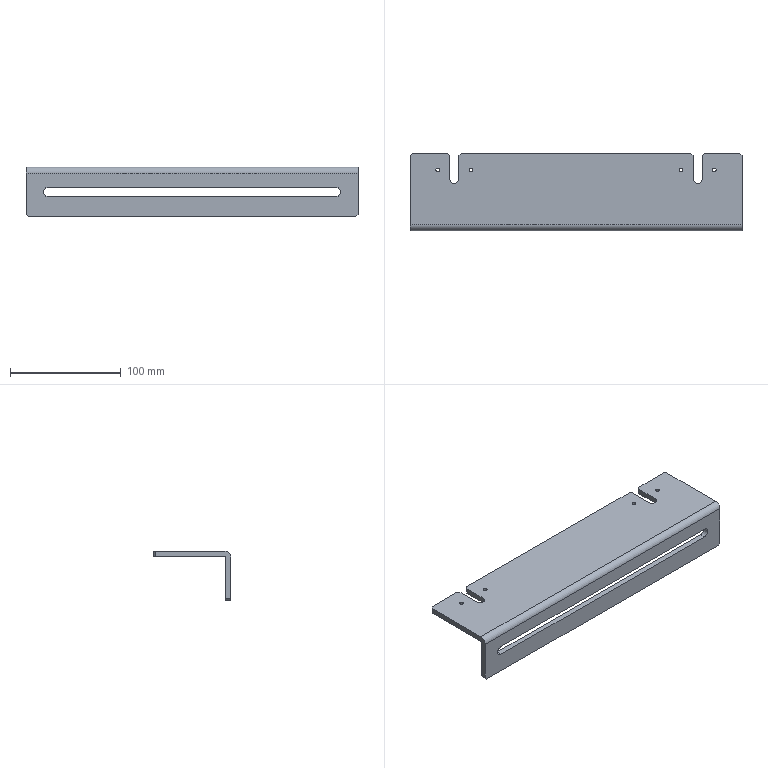Part | SolidWorks | features BaseBody 1 | 1 solid | 38 faces | box 300 x 70 x 45 mm | volume 149245 mm3 | plane 24 | cylinder 14 | commonest cylinder face diameters 3.3 x8 8.5 x4 1 x1 11 x1
STEP:
#1=CARTESIAN_POINT('',(123.35,55.,-5.));
#2=VERTEX_POINT('',#1);
#3=CARTESIAN_POINT('',(126.65,55.,-5.));
#4=VERTEX_POINT('',#3);
#5=CARTESIAN_POINT('',(125.,55.,-5.));
#6=DIRECTION('',(0.,0.,1.));
#7=DIRECTION('',(1.,0.,0.));
#8=AXIS2_PLACEMENT_3D('',#5,#6,#7);
#9=CIRCLE('',#8,1.65);
#10=EDGE_CURVE('',#2,#4,#9,.T.);
#11=ORIENTED_EDGE('',*,*,#10,.F.);
#12=CARTESIAN_POINT('',(123.35,55.,0.));
#13=VERTEX_POINT('',#12);
#14=CARTESIAN_POINT('',(123.35,55.,0.));
#15=DIRECTION('',(0.,0.,1.));
#16=VECTOR('',#15,1000.);
#17=LINE('',#14,#16);
#18=EDGE_CURVE('',#2,#13,#17,.T.);
#19=ORIENTED_EDGE('',*,*,#18,.T.);
#20=CARTESIAN_POINT('',(126.65,55.,0.));
#21=VERTEX_POINT('',#20);
#22=CARTESIAN_POINT('',(125.,55.,0.));
#23=DIRECTION('',(0.,0.,-1.));
#24=DIRECTION('',(1.,0.,0.));
#25=AXIS2_PLACEMENT_3D('',#22,#23,#24);
#26=CIRCLE('',#25,1.65);
#27=EDGE_CURVE('',#21,#13,#26,.T.);
#28=ORIENTED_EDGE('',*,*,#27,.F.);
#29=CARTESIAN_POINT('',(126.65,55.,0.));
#30=DIRECTION('',(0.,0.,1.));
#31=VECTOR('',#30,1000.);
#32=LINE('',#29,#31);
#33=EDGE_CURVE('',#4,#21,#32,.T.);
#34=ORIENTED_EDGE('',*,*,#33,.F.);
#35=EDGE_LOOP('',(#11,#19,#28,#34));
#36=FACE_OUTER_BOUND('',#35,.T.);
#37=CARTESIAN_POINT('',(125.,55.,0.));
#38=DIRECTION('',(0.,0.,1.));
#39=DIRECTION('',(1.,0.,0.));
#40=AXIS2_PLACEMENT_3D('',#37,#38,#39);
#41=CYLINDRICAL_SURFACE('',#40,1.65);
#42=ADVANCED_FACE('',(#36),#41,.F.);
#43=CARTESIAN_POINT('',(93.35,55.,-5.));
#44=VERTEX_POINT('',#43);
#45=CARTESIAN_POINT('',(96.65,55.,-5.));
#46=VERTEX_POINT('',#45);
#47=CARTESIAN_POINT('',(95.,55.,-5.));
#48=DIRECTION('',(0.,0.,1.));
#49=DIRECTION('',(1.,0.,0.));
#50=AXIS2_PLACEMENT_3D('',#47,#48,#49);
#51=CIRCLE('',#50,1.65);
#52=EDGE_CURVE('',#44,#46,#51,.T.);
#53=ORIENTED_EDGE('',*,*,#52,.F.);
#54=CARTESIAN_POINT('',(93.35,55.,0.));
#55=VERTEX_POINT('',#54);
#56=CARTESIAN_POINT('',(93.35,55.,0.));
#57=DIRECTION('',(0.,0.,1.));
#58=VECTOR('',#57,1000.);
#59=LINE('',#56,#58);
#60=EDGE_CURVE('',#44,#55,#59,.T.);
#61=ORIENTED_EDGE('',*,*,#60,.T.);
#62=CARTESIAN_POINT('',(96.65,55.,0.));
#63=VERTEX_POINT('',#62);
#64=CARTESIAN_POINT('',(95.,55.,0.));
#65=DIRECTION('',(0.,0.,-1.));
#66=DIRECTION('',(1.,0.,0.));
#67=AXIS2_PLACEMENT_3D('',#64,#65,#66);
#68=CIRCLE('',#67,1.65);
#69=EDGE_CURVE('',#63,#55,#68,.T.);
#70=ORIENTED_EDGE('',*,*,#69,.F.);
#71=CARTESIAN_POINT('',(96.65,55.,0.));
#72=DIRECTION('',(0.,0.,1.));
#73=VECTOR('',#72,1000.);
#74=LINE('',#71,#73);
#75=EDGE_CURVE('',#46,#63,#74,.T.);
#76=ORIENTED_EDGE('',*,*,#75,.F.);
#77=EDGE_LOOP('',(#53,#61,#70,#76));
#78=FACE_OUTER_BOUND('',#77,.T.);
#79=CARTESIAN_POINT('',(95.,55.,0.));
#80=DIRECTION('',(0.,0.,1.));
#81=DIRECTION('',(1.,0.,0.));
#82=AXIS2_PLACEMENT_3D('',#79,#80,#81);
#83=CYLINDRICAL_SURFACE('',#82,1.65);
#84=ADVANCED_FACE('',(#78),#83,.F.);
#85=CARTESIAN_POINT('',(-126.65,55.,-5.));
#86=VERTEX_POINT('',#85);
#87=CARTESIAN_POINT('',(-123.35,55.,-5.));
#88=VERTEX_POINT('',#87);
#89=CARTESIAN_POINT('',(-125.,55.,-5.));
#90=DIRECTION('',(0.,0.,1.));
#91=DIRECTION('',(1.,0.,0.));
#92=AXIS2_PLACEMENT_3D('',#89,#90,#91);
#93=CIRCLE('',#92,1.65);
#94=EDGE_CURVE('',#86,#88,#93,.T.);
#95=ORIENTED_EDGE('',*,*,#94,.F.);
#96=CARTESIAN_POINT('',(-126.65,55.,0.));
#97=VERTEX_POINT('',#96);
#98=CARTESIAN_POINT('',(-126.65,55.,0.));
#99=DIRECTION('',(0.,0.,1.));
#100=VECTOR('',#99,1000.);
#101=LINE('',#98,#100);
#102=EDGE_CURVE('',#86,#97,#101,.T.);
#103=ORIENTED_EDGE('',*,*,#102,.T.);
#104=CARTESIAN_POINT('',(-123.35,55.,0.));
#105=VERTEX_POINT('',#104);
#106=CARTESIAN_POINT('',(-125.,55.,0.));
#107=DIRECTION('',(0.,0.,-1.));
#108=DIRECTION('',(1.,0.,0.));
#109=AXIS2_PLACEMENT_3D('',#106,#107,#108);
#110=CIRCLE('',#109,1.65);
#111=EDGE_CURVE('',#105,#97,#110,.T.);
#112=ORIENTED_EDGE('',*,*,#111,.F.);
#113=CARTESIAN_POINT('',(-123.35,55.,0.));
#114=DIRECTION('',(0.,0.,1.));
#115=VECTOR('',#114,1000.);
#116=LINE('',#113,#115);
#117=EDGE_CURVE('',#88,#105,#116,.T.);
#118=ORIENTED_EDGE('',*,*,#117,.F.);
#119=EDGE_LOOP('',(#95,#103,#112,#118));
#120=FACE_OUTER_BOUND('',#119,.T.);
#121=CARTESIAN_POINT('',(-125.,55.,0.));
#122=DIRECTION('',(0.,0.,1.));
#123=DIRECTION('',(1.,0.,0.));
#124=AXIS2_PLACEMENT_3D('',#121,#122,#123);
#125=CYLINDRICAL_SURFACE('',#124,1.65);
#126=ADVANCED_FACE('',(#120),#125,.F.);
#127=CARTESIAN_POINT('',(-96.65,55.,-5.));
#128=VERTEX_POINT('',#127);
#129=CARTESIAN_POINT('',(-93.35,55.,-5.));
#130=VERTEX_POINT('',#129);
#131=CARTESIAN_POINT('',(-95.,55.,-5.));
#132=DIRECTION('',(0.,0.,1.));
#133=DIRECTION('',(1.,0.,0.));
#134=AXIS2_PLACEMENT_3D('',#131,#132,#133);
#135=CIRCLE('',#134,1.65);
#136=EDGE_CURVE('',#128,#130,#135,.T.);
#137=ORIENTED_EDGE('',*,*,#136,.F.);
#138=CARTESIAN_POINT('',(-96.65,55.,0.));
#139=VERTEX_POINT('',#138);
#140=CARTESIAN_POINT('',(-96.65,55.,0.));
#141=DIRECTION('',(0.,0.,1.));
#142=VECTOR('',#141,1000.);
#143=LINE('',#140,#142);
#144=EDGE_CURVE('',#128,#139,#143,.T.);
#145=ORIENTED_EDGE('',*,*,#144,.T.);
#146=CARTESIAN_POINT('',(-93.35,55.,0.));
#147=VERTEX_POINT('',#146);
#148=CARTESIAN_POINT('',(-95.,55.,0.));
#149=DIRECTION('',(0.,0.,-1.));
#150=DIRECTION('',(1.,0.,0.));
#151=AXIS2_PLACEMENT_3D('',#148,#149,#150);
#152=CIRCLE('',#151,1.65);
#153=EDGE_CURVE('',#147,#139,#152,.T.);
#154=ORIENTED_EDGE('',*,*,#153,.F.);
#155=CARTESIAN_POINT('',(-93.35,55.,0.));
#156=DIRECTION('',(0.,0.,1.));
#157=VECTOR('',#156,1000.);
#158=LINE('',#155,#157);
#159=EDGE_CURVE('',#130,#147,#158,.T.);
#160=ORIENTED_EDGE('',*,*,#159,.F.);
#161=EDGE_LOOP('',(#137,#145,#154,#160));
#162=FACE_OUTER_BOUND('',#161,.T.);
#163=CARTESIAN_POINT('',(-95.,55.,0.));
#164=DIRECTION('',(0.,0.,1.));
#165=DIRECTION('',(1.,0.,0.));
#166=AXIS2_PLACEMENT_3D('',#163,#164,#165);
#167=CYLINDRICAL_SURFACE('',#166,1.65);
#168=ADVANCED_FACE('',(#162),#167,.F.);
#169=CARTESIAN_POINT('',(125.,55.,-5.));
#170=DIRECTION('',(0.,0.,1.));
#171=DIRECTION('',(1.,0.,0.));
#172=AXIS2_PLACEMENT_3D('',#169,#170,#171);
#173=CIRCLE('',#172,1.65);
#174=EDGE_CURVE('',#4,#2,#173,.T.);
#175=ORIENTED_EDGE('',*,*,#174,.T.);
#176=ORIENTED_EDGE('',*,*,#10,.T.);
#177=EDGE_LOOP('',(#175,#176));
#178=FACE_BOUND('',#177,.T.);
#179=CARTESIAN_POINT('',(95.,55.,-5.));
#180=DIRECTION('',(0.,0.,1.));
#181=DIRECTION('',(1.,0.,0.));
#182=AXIS2_PLACEMENT_3D('',#179,#180,#181);
#183=CIRCLE('',#182,1.65);
#184=EDGE_CURVE('',#46,#44,#183,.T.);
#185=ORIENTED_EDGE('',*,*,#184,.T.);
#186=ORIENTED_EDGE('',*,*,#52,.T.);
#187=EDGE_LOOP('',(#185,#186));
#188=FACE_BOUND('',#187,.T.);
#189=CARTESIAN_POINT('',(-114.25,68.,-5.));
#190=VERTEX_POINT('',#189);
#191=CARTESIAN_POINT('',(-114.25,47.,-5.));
#192=VERTEX_POINT('',#191);
#193=CARTESIAN_POINT('',(-114.25,0.,-5.));
#194=DIRECTION('',(0.,-1.,0.));
#195=VECTOR('',#194,1000.);
#196=LINE('',#193,#195);
#197=EDGE_CURVE('',#190,#192,#196,.T.);
#198=ORIENTED_EDGE('',*,*,#197,.T.);
#199=CARTESIAN_POINT('',(-105.75,47.,-5.));
#200=VERTEX_POINT('',#199);
#201=CARTESIAN_POINT('',(-110.,47.,-5.));
#202=DIRECTION('',(0.,0.,1.));
#203=DIRECTION('',(1.,0.,0.));
#204=AXIS2_PLACEMENT_3D('',#201,#202,#203);
#205=CIRCLE('',#204,4.25);
#206=EDGE_CURVE('',#192,#200,#205,.T.);
#207=ORIENTED_EDGE('',*,*,#206,.T.);
#208=CARTESIAN_POINT('',(-105.75,68.,-5.));
#209=VERTEX_POINT('',#208);
#210=CARTESIAN_POINT('',(-105.75,0.,-5.));
#211=DIRECTION('',(0.,1.,0.));
#212=VECTOR('',#211,1000.);
#213=LINE('',#210,#212);
#214=EDGE_CURVE('',#200,#209,#213,.T.);
#215=ORIENTED_EDGE('',*,*,#214,.T.);
#216=CARTESIAN_POINT('',(-103.75,70.,-5.));
#217=VERTEX_POINT('',#216);
#218=CARTESIAN_POINT('',(-105.75,68.,-5.));
#219=DIRECTION('',(0.7071,0.7071,0.));
#220=VECTOR('',#219,1000.);
#221=LINE('',#218,#220);
#222=EDGE_CURVE('',#209,#217,#221,.T.);
#223=ORIENTED_EDGE('',*,*,#222,.T.);
#224=CARTESIAN_POINT('',(103.75,70.,-5.));
#225=VERTEX_POINT('',#224);
#226=CARTESIAN_POINT('',(-150.,70.,-5.));
#227=DIRECTION('',(1.,0.,0.));
#228=VECTOR('',#227,1000.);
#229=LINE('',#226,#228);
#230=EDGE_CURVE('',#217,#225,#229,.T.);
#231=ORIENTED_EDGE('',*,*,#230,.T.);
#232=CARTESIAN_POINT('',(105.75,68.,-5.));
#233=VERTEX_POINT('',#232);
#234=CARTESIAN_POINT('',(103.75,70.,-5.));
#235=DIRECTION('',(0.7071,-0.7071,0.));
#236=VECTOR('',#235,1000.);
#237=LINE('',#234,#236);
#238=EDGE_CURVE('',#225,#233,#237,.T.);
#239=ORIENTED_EDGE('',*,*,#238,.T.);
#240=CARTESIAN_POINT('',(105.75,47.,-5.));
#241=VERTEX_POINT('',#240);
#242=CARTESIAN_POINT('',(105.75,0.,-5.));
#243=DIRECTION('',(0.,-1.,0.));
#244=VECTOR('',#243,1000.);
#245=LINE('',#242,#244);
#246=EDGE_CURVE('',#233,#241,#245,.T.);
#247=ORIENTED_EDGE('',*,*,#246,.T.);
#248=CARTESIAN_POINT('',(114.25,47.,-5.));
#249=VERTEX_POINT('',#248);
#250=CARTESIAN_POINT('',(110.,47.,-5.));
#251=DIRECTION('',(0.,0.,1.));
#252=DIRECTION('',(1.,0.,0.));
#253=AXIS2_PLACEMENT_3D('',#250,#251,#252);
#254=CIRCLE('',#253,4.25);
#255=EDGE_CURVE('',#241,#249,#254,.T.);
#256=ORIENTED_EDGE('',*,*,#255,.T.);
#257=CARTESIAN_POINT('',(114.25,68.,-5.));
#258=VERTEX_POINT('',#257);
#259=CARTESIAN_POINT('',(114.25,0.,-5.));
#260=DIRECTION('',(0.,1.,0.));
#261=VECTOR('',#260,1000.);
#262=LINE('',#259,#261);
#263=EDGE_CURVE('',#249,#258,#262,.T.);
#264=ORIENTED_EDGE('',*,*,#263,.T.);
#265=CARTESIAN_POINT('',(116.25,70.,-5.));
#266=VERTEX_POINT('',#265);
#267=CARTESIAN_POINT('',(114.25,68.,-5.));
#268=DIRECTION('',(0.7071,0.7071,0.));
#269=VECTOR('',#268,1000.);
#270=LINE('',#267,#269);
#271=EDGE_CURVE('',#258,#266,#270,.T.);
#272=ORIENTED_EDGE('',*,*,#271,.T.);
#273=CARTESIAN_POINT('',(148.,70.,-5.));
#274=VERTEX_POINT('',#273);
#275=CARTESIAN_POINT('',(-150.,70.,-5.));
#276=DIRECTION('',(1.,0.,0.));
#277=VECTOR('',#276,1000.);
#278=LINE('',#275,#277);
#279=EDGE_CURVE('',#266,#274,#278,.T.);
#280=ORIENTED_EDGE('',*,*,#279,.T.);
#281=CARTESIAN_POINT('',(150.,68.,-5.));
#282=VERTEX_POINT('',#281);
#283=CARTESIAN_POINT('',(148.,70.,-5.));
#284=DIRECTION('',(0.7071,-0.7071,0.));
#285=VECTOR('',#284,1000.);
#286=LINE('',#283,#285);
#287=EDGE_CURVE('',#274,#282,#286,.T.);
#288=ORIENTED_EDGE('',*,*,#287,.T.);
#289=CARTESIAN_POINT('',(150.,5.5,-5.));
#290=VERTEX_POINT('',#289);
#291=CARTESIAN_POINT('',(150.,0.,-5.));
#292=DIRECTION('',(0.,-1.,0.));
#293=VECTOR('',#292,1000.);
#294=LINE('',#291,#293);
#295=EDGE_CURVE('',#282,#290,#294,.T.);
#296=ORIENTED_EDGE('',*,*,#295,.T.);
#297=CARTESIAN_POINT('',(-150.,5.5,-5.));
#298=VERTEX_POINT('',#297);
#299=CARTESIAN_POINT('',(-150.,5.5,-5.));
#300=DIRECTION('',(-1.,0.,0.));
#301=VECTOR('',#300,1000.);
#302=LINE('',#299,#301);
#303=EDGE_CURVE('',#290,#298,#302,.T.);
#304=ORIENTED_EDGE('',*,*,#303,.T.);
#305=CARTESIAN_POINT('',(-150.,68.,-5.));
#306=VERTEX_POINT('',#305);
#307=CARTESIAN_POINT('',(-150.,0.,-5.));
#308=DIRECTION('',(0.,1.,0.));
#309=VECTOR('',#308,1000.);
#310=LINE('',#307,#309);
#311=EDGE_CURVE('',#298,#306,#310,.T.);
#312=ORIENTED_EDGE('',*,*,#311,.T.);
#313=CARTESIAN_POINT('',(-148.,70.,-5.));
#314=VERTEX_POINT('',#313);
#315=CARTESIAN_POINT('',(-150.,68.,-5.));
#316=DIRECTION('',(0.7071,0.7071,0.));
#317=VECTOR('',#316,1000.);
#318=LINE('',#315,#317);
#319=EDGE_CURVE('',#306,#314,#318,.T.);
#320=ORIENTED_EDGE('',*,*,#319,.T.);
#321=CARTESIAN_POINT('',(-116.25,70.,-5.));
#322=VERTEX_POINT('',#321);
#323=CARTESIAN_POINT('',(-150.,70.,-5.));
#324=DIRECTION('',(1.,0.,0.));
#325=VECTOR('',#324,1000.);
#326=LINE('',#323,#325);
#327=EDGE_CURVE('',#314,#322,#326,.T.);
#328=ORIENTED_EDGE('',*,*,#327,.T.);
#329=CARTESIAN_POINT('',(-116.25,70.,-5.));
#330=DIRECTION('',(0.7071,-0.7071,0.));
#331=VECTOR('',#330,1000.);
#332=LINE('',#329,#331);
#333=EDGE_CURVE('',#322,#190,#332,.T.);
#334=ORIENTED_EDGE('',*,*,#333,.T.);
#335=EDGE_LOOP('',(#198,#207,#215,#223,#231,#239,#247,#256,#264,#272,#280,#288,#296,#304,#312,#320,#328,#334));
#336=FACE_OUTER_BOUND('',#335,.T.);
#337=CARTESIAN_POINT('',(-125.,55.,-5.));
#338=DIRECTION('',(0.,0.,1.));
#339=DIRECTION('',(1.,0.,0.));
#340=AXIS2_PLACEMENT_3D('',#337,#338,#339);
#341=CIRCLE('',#340,1.65);
#342=EDGE_CURVE('',#88,#86,#341,.T.);
#343=ORIENTED_EDGE('',*,*,#342,.T.);
#344=ORIENTED_EDGE('',*,*,#94,.T.);
#345=EDGE_LOOP('',(#343,#344));
#346=FACE_BOUND('',#345,.T.);
#347=CARTESIAN_POINT('',(-95.,55.,-5.));
#348=DIRECTION('',(0.,0.,1.));
#349=DIRECTION('',(1.,0.,0.));
#350=AXIS2_PLACEMENT_3D('',#347,#348,#349);
#351=CIRCLE('',#350,1.65);
#352=EDGE_CURVE('',#130,#128,#351,.T.);
#353=ORIENTED_EDGE('',*,*,#352,.T.);
#354=ORIENTED_EDGE('',*,*,#136,.T.);
#355=EDGE_LOOP('',(#353,#354));
#356=FACE_BOUND('',#355,.T.);
#357=CARTESIAN_POINT('',(-150.,0.,-5.));
#358=DIRECTION('',(0.,0.,-1.));
#359=DIRECTION('',(-1.,0.,0.));
#360=AXIS2_PLACEMENT_3D('',#357,#358,#359);
#361=PLANE('',#360);
#362=ADVANCED_FACE('',(#178,#188,#336,#346,#356),#361,.T.);
#363=ORIENTED_EDGE('',*,*,#18,.F.);
#364=ORIENTED_EDGE('',*,*,#174,.F.);
#365=ORIENTED_EDGE('',*,*,#33,.T.);
#366=CARTESIAN_POINT('',(125.,55.,0.));
#367=DIRECTION('',(0.,0.,-1.));
#368=DIRECTION('',(1.,0.,0.));
#369=AXIS2_PLACEMENT_3D('',#366,#367,#368);
#370=CIRCLE('',#369,1.65);
#371=EDGE_CURVE('',#13,#21,#370,.T.);
#372=ORIENTED_EDGE('',*,*,#371,.F.);
#373=EDGE_LOOP('',(#363,#364,#365,#372));
#374=FACE_OUTER_BOUND('',#373,.T.);
#375=CARTESIAN_POINT('',(125.,55.,0.));
#376=DIRECTION('',(0.,0.,1.));
#377=DIRECTION('',(1.,0.,0.));
#378=AXIS2_PLACEMENT_3D('',#375,#376,#377);
#379=CYLINDRICAL_SURFACE('',#378,1.65);
#380=ADVANCED_FACE('',(#374),#379,.F.);
#381=ORIENTED_EDGE('',*,*,#60,.F.);
#382=ORIENTED_EDGE('',*,*,#184,.F.);
#383=ORIENTED_EDGE('',*,*,#75,.T.);
#384=CARTESIAN_POINT('',(95.,55.,0.));
#385=DIRECTION('',(0.,0.,-1.));
#386=DIRECTION('',(1.,0.,0.));
#387=AXIS2_PLACEMENT_3D('',#384,#385,#386);
#388=CIRCLE('',#387,1.65);
#389=EDGE_CURVE('',#55,#63,#388,.T.);
#390=ORIENTED_EDGE('',*,*,#389,.F.);
#391=EDGE_LOOP('',(#381,#382,#383,#390));
#392=FACE_OUTER_BOUND('',#391,.T.);
#393=CARTESIAN_POINT('',(95.,55.,0.));
#394=DIRECTION('',(0.,0.,1.));
#395=DIRECTION('',(1.,0.,0.));
#396=AXIS2_PLACEMENT_3D('',#393,#394,#395);
#397=CYLINDRICAL_SURFACE('',#396,1.65);
#398=ADVANCED_FACE('',(#392),#397,.F.);
#399=CARTESIAN_POINT('',(-114.25,47.,0.));
#400=VERTEX_POINT('',#399);
#401=CARTESIAN_POINT('',(-114.25,47.,-45.));
#402=DIRECTION('',(0.,0.,-1.));
#403=VECTOR('',#402,1000.);
#404=LINE('',#401,#403);
#405=EDGE_CURVE('',#400,#192,#404,.T.);
#406=ORIENTED_EDGE('',*,*,#405,.F.);
#407=CARTESIAN_POINT('',(-105.75,47.,0.));
#408=VERTEX_POINT('',#407);
#409=CARTESIAN_POINT('',(-110.,47.,0.));
#410=DIRECTION('',(0.,0.,-1.));
#411=DIRECTION('',(1.,0.,0.));
#412=AXIS2_PLACEMENT_3D('',#409,#410,#411);
#413=CIRCLE('',#412,4.25);
#414=EDGE_CURVE('',#408,#400,#413,.T.);
#415=ORIENTED_EDGE('',*,*,#414,.F.);
#416=CARTESIAN_POINT('',(-105.75,47.,-45.));
#417=DIRECTION('',(0.,0.,1.));
#418=VECTOR('',#417,1000.);
#419=LINE('',#416,#418);
#420=EDGE_CURVE('',#200,#408,#419,.T.);
#421=ORIENTED_EDGE('',*,*,#420,.F.);
#422=ORIENTED_EDGE('',*,*,#206,.F.);
#423=EDGE_LOOP('',(#406,#415,#421,#422));
#424=FACE_OUTER_BOUND('',#423,.T.);
#425=CARTESIAN_POINT('',(-110.,47.,-45.));
#426=DIRECTION('',(0.,0.,1.));
#427=DIRECTION('',(1.,0.,0.));
#428=AXIS2_PLACEMENT_3D('',#425,#426,#427);
#429=CYLINDRICAL_SURFACE('',#428,4.25);
#430=ADVANCED_FACE('',(#424),#429,.F.);
#431=CARTESIAN_POINT('',(-114.25,68.,0.));
#432=VERTEX_POINT('',#431);
#433=CARTESIAN_POINT('',(-114.25,68.,-45.));
#434=DIRECTION('',(0.,0.,-1.));
#435=VECTOR('',#434,1000.);
#436=LINE('',#433,#435);
#437=EDGE_CURVE('',#432,#190,#436,.T.);
#438=ORIENTED_EDGE('',*,*,#437,.F.);
#439=CARTESIAN_POINT('',(-114.25,93.,0.));
#440=DIRECTION('',(0.,1.,0.));
#441=VECTOR('',#440,1000.);
#442=LINE('',#439,#441);
#443=EDGE_CURVE('',#400,#432,#442,.T.);
#444=ORIENTED_EDGE('',*,*,#443,.F.);
#445=ORIENTED_EDGE('',*,*,#405,.T.);
#446=ORIENTED_EDGE('',*,*,#197,.F.);
#447=EDGE_LOOP('',(#438,#444,#445,#446));
#448=FACE_OUTER_BOUND('',#447,.T.);
#449=CARTESIAN_POINT('',(-114.25,93.,-45.));
#450=DIRECTION('',(-1.,0.,0.));
#451=DIRECTION('',(0.,0.,1.));
#452=AXIS2_PLACEMENT_3D('',#449,#450,#451);
#453=PLANE('',#452);
#454=ADVANCED_FACE('',(#448),#453,.F.);
#455=ORIENTED_EDGE('',*,*,#437,.T.);
#456=ORIENTED_EDGE('',*,*,#333,.F.);
#457=CARTESIAN_POINT('',(-116.25,70.,0.));
#458=VERTEX_POINT('',#457);
#459=CARTESIAN_POINT('',(-116.25,70.,0.));
#460=DIRECTION('',(0.,0.,-1.));
#461=VECTOR('',#460,1000.);
#462=LINE('',#459,#461);
#463=EDGE_CURVE('',#458,#322,#462,.T.);
#464=ORIENTED_EDGE('',*,*,#463,.F.);
#465=CARTESIAN_POINT('',(-116.25,70.,0.));
#466=DIRECTION('',(-0.7071,0.7071,0.));
#467=VECTOR('',#466,1000.);
#468=LINE('',#465,#467);
#469=EDGE_CURVE('',#432,#458,#468,.T.);
#470=ORIENTED_EDGE('',*,*,#469,.F.);
#471=EDGE_LOOP('',(#455,#456,#464,#470));
#472=FACE_OUTER_BOUND('',#471,.T.);
#473=CARTESIAN_POINT('',(-116.25,70.,0.));
#474=DIRECTION('',(-0.7071,-0.7071,0.));
#475=DIRECTION('',(0.7071,-0.7071,0.));
#476=AXIS2_PLACEMENT_3D('',#473,#474,#475);
#477=PLANE('',#476);
#478=ADVANCED_FACE('',(#472),#477,.F.);
#479=ORIENTED_EDGE('',*,*,#463,.T.);
#480=ORIENTED_EDGE('',*,*,#327,.F.);
#481=CARTESIAN_POINT('',(-148.,70.,0.));
#482=VERTEX_POINT('',#481);
#483=CARTESIAN_POINT('',(-148.,70.,0.));
#484=DIRECTION('',(0.,0.,-1.));
#485=VECTOR('',#484,1000.);
#486=LINE('',#483,#485);
#487=EDGE_CURVE('',#482,#314,#486,.T.);
#488=ORIENTED_EDGE('',*,*,#487,.F.);
#489=CARTESIAN_POINT('',(-150.,70.,0.));
#490=DIRECTION('',(-1.,0.,0.));
#491=VECTOR('',#490,1000.);
#492=LINE('',#489,#491);
#493=EDGE_CURVE('',#458,#482,#492,.T.);
#494=ORIENTED_EDGE('',*,*,#493,.F.);
#495=EDGE_LOOP('',(#479,#480,#488,#494));
#496=FACE_OUTER_BOUND('',#495,.T.);
#497=CARTESIAN_POINT('',(-150.,70.,0.));
#498=DIRECTION('',(0.,-1.,0.));
#499=DIRECTION('',(0.,0.,-1.));
#500=AXIS2_PLACEMENT_3D('',#497,#498,#499);
#501=PLANE('',#500);
#502=ADVANCED_FACE('',(#496),#501,.F.);
#503=ORIENTED_EDGE('',*,*,#487,.T.);
#504=ORIENTED_EDGE('',*,*,#319,.F.);
#505=CARTESIAN_POINT('',(-150.,68.,0.));
#506=VERTEX_POINT('',#505);
#507=CARTESIAN_POINT('',(-150.,68.,-5.5));
#508=DIRECTION('',(0.,0.,-1.));
#509=VECTOR('',#508,1000.);
#510=LINE('',#507,#509);
#511=EDGE_CURVE('',#506,#306,#510,.T.);
#512=ORIENTED_EDGE('',*,*,#511,.F.);
#513=CARTESIAN_POINT('',(-150.,68.,0.));
#514=DIRECTION('',(-0.7071,-0.7071,0.));
#515=VECTOR('',#514,1000.);
#516=LINE('',#513,#515);
#517=EDGE_CURVE('',#482,#506,#516,.T.);
#518=ORIENTED_EDGE('',*,*,#517,.F.);
#519=EDGE_LOOP('',(#503,#504,#512,#518));
#520=FACE_OUTER_BOUND('',#519,.T.);
#521=CARTESIAN_POINT('',(-150.,68.,-5.5));
#522=DIRECTION('',(0.7071,-0.7071,0.));
#523=DIRECTION('',(0.7071,0.7071,0.));
#524=AXIS2_PLACEMENT_3D('',#521,#522,#523);
#525=PLANE('',#524);
#526=ADVANCED_FACE('',(#520),#525,.F.);
#527=ORIENTED_EDGE('',*,*,#511,.T.);
#528=ORIENTED_EDGE('',*,*,#311,.F.);
#529=CARTESIAN_POINT('',(-150.,5.,-5.5));
#530=VERTEX_POINT('',#529);
#531=CARTESIAN_POINT('',(-150.,5.5,-5.5));
#532=DIRECTION('',(1.,0.,0.));
#533=DIRECTION('',(0.,0.,-1.));
#534=AXIS2_PLACEMENT_3D('',#531,#532,#533);
#535=CIRCLE('',#534,0.5);
#536=EDGE_CURVE('',#298,#530,#535,.T.);
#537=ORIENTED_EDGE('',*,*,#536,.T.);
#538=CARTESIAN_POINT('',(-150.,5.,-43.));
#539=VERTEX_POINT('',#538);
#540=CARTESIAN_POINT('',(-150.,5.,-45.));
#541=DIRECTION('',(0.,0.,1.));
#542=VECTOR('',#541,1000.);
#543=LINE('',#540,#542);
#544=EDGE_CURVE('',#539,#530,#543,.T.);
#545=ORIENTED_EDGE('',*,*,#544,.F.);
#546=CARTESIAN_POINT('',(-150.,0.,-43.));
#547=VERTEX_POINT('',#546);
#548=CARTESIAN_POINT('',(-150.,5.5,-43.));
#549=DIRECTION('',(0.,-1.,0.));
#550=VECTOR('',#549,1000.);
#551=LINE('',#548,#550);
#552=EDGE_CURVE('',#539,#547,#551,.T.);
#553=ORIENTED_EDGE('',*,*,#552,.T.);
#554=CARTESIAN_POINT('',(-150.,0.,-5.5));
#555=VERTEX_POINT('',#554);
#556=CARTESIAN_POINT('',(-150.,0.,-5.));
#557=DIRECTION('',(0.,0.,1.));
#558=VECTOR('',#557,1000.);
#559=LINE('',#556,#558);
#560=EDGE_CURVE('',#547,#555,#559,.T.);
#561=ORIENTED_EDGE('',*,*,#560,.T.);
#562=CARTESIAN_POINT('',(-150.,5.5,0.));
#563=VERTEX_POINT('',#562);
#564=CARTESIAN_POINT('',(-150.,5.5,-5.5));
#565=DIRECTION('',(-1.,0.,0.));
#566=DIRECTION('',(0.,0.,-1.));
#567=AXIS2_PLACEMENT_3D('',#564,#565,#566);
#568=CIRCLE('',#567,5.5);
#569=EDGE_CURVE('',#555,#563,#568,.T.);
#570=ORIENTED_EDGE('',*,*,#569,.T.);
#571=CARTESIAN_POINT('',(-150.,5.5,0.));
#572=DIRECTION('',(0.,-1.,0.));
#573=VECTOR('',#572,1000.);
#574=LINE('',#571,#573);
#575=EDGE_CURVE('',#506,#563,#574,.T.);
#576=ORIENTED_EDGE('',*,*,#575,.F.);
#577=EDGE_LOOP('',(#527,#528,#537,#545,#553,#561,#570,#576));
#578=FACE_OUTER_BOUND('',#577,.T.);
#579=CARTESIAN_POINT('',(-150.,5.5,-5.5));
#580=DIRECTION('',(1.,0.,0.));
#581=DIRECTION('',(0.,0.,-1.));
#582=AXIS2_PLACEMENT_3D('',#579,#580,#581);
#583=PLANE('',#582);
#584=ADVANCED_FACE('',(#578),#583,.F.);
#585=CARTESIAN_POINT('',(150.,5.,-5.5));
#586=VERTEX_POINT('',#585);
#587=CARTESIAN_POINT('',(-150.,5.,-5.5));
#588=DIRECTION('',(1.,0.,0.));
#589=VECTOR('',#588,1000.);
#590=LINE('',#587,#589);
#591=EDGE_CURVE('',#530,#586,#590,.T.);
#592=ORIENTED_EDGE('',*,*,#591,.F.);
#593=ORIENTED_EDGE('',*,*,#536,.F.);
#594=ORIENTED_EDGE('',*,*,#303,.F.);
#595=CARTESIAN_POINT('',(150.,5.5,-5.5));
#596=DIRECTION('',(-1.,0.,0.));
#597=DIRECTION('',(0.,0.,-1.));
#598=AXIS2_PLACEMENT_3D('',#595,#596,#597);
#599=CIRCLE('',#598,0.5);
#600=EDGE_CURVE('',#586,#290,#599,.T.);
#601=ORIENTED_EDGE('',*,*,#600,.F.);
#602=EDGE_LOOP('',(#592,#593,#594,#601));
#603=FACE_OUTER_BOUND('',#602,.T.);
#604=CARTESIAN_POINT('',(-150.,5.5,-5.5));
#605=DIRECTION('',(1.,0.,0.));
#606=DIRECTION('',(0.,0.,-1.));
#607=AXIS2_PLACEMENT_3D('',#604,#605,#606);
#608=CYLINDRICAL_SURFACE('',#607,0.5);
#609=ADVANCED_FACE('',(#603),#608,.F.);
#610=CARTESIAN_POINT('',(150.,68.,0.));
#611=VERTEX_POINT('',#610);
#612=CARTESIAN_POINT('',(150.,5.5,0.));
#613=VERTEX_POINT('',#612);
#614=CARTESIAN_POINT('',(150.,5.,0.));
#615=DIRECTION('',(0.,-1.,0.));
#616=VECTOR('',#615,1000.);
#617=LINE('',#614,#616);
#618=EDGE_CURVE('',#611,#613,#617,.T.);
#619=ORIENTED_EDGE('',*,*,#618,.T.);
#620=CARTESIAN_POINT('',(150.,0.,-5.5));
#621=VERTEX_POINT('',#620);
#622=CARTESIAN_POINT('',(150.,5.5,-5.5));
#623=DIRECTION('',(1.,0.,0.));
#624=DIRECTION('',(0.,0.,-1.));
#625=AXIS2_PLACEMENT_3D('',#622,#623,#624);
#626=CIRCLE('',#625,5.5);
#627=EDGE_CURVE('',#613,#621,#626,.T.);
#628=ORIENTED_EDGE('',*,*,#627,.T.);
#629=CARTESIAN_POINT('',(150.,0.,-43.));
#630=VERTEX_POINT('',#629);
#631=CARTESIAN_POINT('',(150.,0.,-5.5));
#632=DIRECTION('',(0.,0.,-1.));
#633=VECTOR('',#632,1000.);
#634=LINE('',#631,#633);
#635=EDGE_CURVE('',#621,#630,#634,.T.);
#636=ORIENTED_EDGE('',*,*,#635,.T.);
#637=CARTESIAN_POINT('',(150.,5.,-43.));
#638=VERTEX_POINT('',#637);
#639=CARTESIAN_POINT('',(150.,5.,-43.));
#640=DIRECTION('',(0.,-1.,0.));
#641=VECTOR('',#640,1000.);
#642=LINE('',#639,#641);
#643=EDGE_CURVE('',#638,#630,#642,.T.);
#644=ORIENTED_EDGE('',*,*,#643,.F.);
#645=CARTESIAN_POINT('',(150.,5.,-45.));
#646=DIRECTION('',(0.,0.,-1.));
#647=VECTOR('',#646,1000.);
#648=LINE('',#645,#647);
#649=EDGE_CURVE('',#586,#638,#648,.T.);
#650=ORIENTED_EDGE('',*,*,#649,.F.);
#651=ORIENTED_EDGE('',*,*,#600,.T.);
#652=ORIENTED_EDGE('',*,*,#295,.F.);
#653=CARTESIAN_POINT('',(150.,68.,-5.5));
#654=DIRECTION('',(0.,0.,1.));
#655=VECTOR('',#654,1000.);
#656=LINE('',#653,#655);
#657=EDGE_CURVE('',#282,#611,#656,.T.);
#658=ORIENTED_EDGE('',*,*,#657,.T.);
#659=EDGE_LOOP('',(#619,#628,#636,#644,#650,#651,#652,#658));
#660=FACE_OUTER_BOUND('',#659,.T.);
#661=CARTESIAN_POINT('',(150.,5.,-5.5));
#662=DIRECTION('',(1.,0.,0.));
#663=DIRECTION('',(0.,0.,-1.));
#664=AXIS2_PLACEMENT_3D('',#661,#662,#663);
#665=PLANE('',#664);
#666=ADVANCED_FACE('',(#660),#665,.T.);
#667=ORIENTED_EDGE('',*,*,#287,.F.);
#668=CARTESIAN_POINT('',(148.,70.,0.));
#669=VERTEX_POINT('',#668);
#670=CARTESIAN_POINT('',(148.,70.,0.));
#671=DIRECTION('',(0.,0.,1.));
#672=VECTOR('',#671,1000.);
#673=LINE('',#670,#672);
#674=EDGE_CURVE('',#274,#669,#673,.T.);
#675=ORIENTED_EDGE('',*,*,#674,.T.);
#676=CARTESIAN_POINT('',(148.,70.,0.));
#677=DIRECTION('',(0.7071,-0.7071,0.));
#678=VECTOR('',#677,1000.);
#679=LINE('',#676,#678);
#680=EDGE_CURVE('',#669,#611,#679,.T.);
#681=ORIENTED_EDGE('',*,*,#680,.T.);
#682=ORIENTED_EDGE('',*,*,#657,.F.);
#683=EDGE_LOOP('',(#667,#675,#681,#682));
#684=FACE_OUTER_BOUND('',#683,.T.);
#685=CARTESIAN_POINT('',(148.,70.,0.));
#686=DIRECTION('',(0.7071,0.7071,0.));
#687=DIRECTION('',(-0.7071,0.7071,0.));
#688=AXIS2_PLACEMENT_3D('',#685,#686,#687);
#689=PLANE('',#688);
#690=ADVANCED_FACE('',(#684),#689,.T.);
#691=ORIENTED_EDGE('',*,*,#674,.F.);
#692=ORIENTED_EDGE('',*,*,#279,.F.);
#693=CARTESIAN_POINT('',(116.25,70.,0.));
#694=VERTEX_POINT('',#693);
#695=CARTESIAN_POINT('',(116.25,70.,0.));
#696=DIRECTION('',(0.,0.,-1.));
#697=VECTOR('',#696,1000.);
#698=LINE('',#695,#697);
#699=EDGE_CURVE('',#694,#266,#698,.T.);
#700=ORIENTED_EDGE('',*,*,#699,.F.);
#701=CARTESIAN_POINT('',(-150.,70.,0.));
#702=DIRECTION('',(-1.,0.,0.));
#703=VECTOR('',#702,1000.);
#704=LINE('',#701,#703);
#705=EDGE_CURVE('',#669,#694,#704,.T.);
#706=ORIENTED_EDGE('',*,*,#705,.F.);
#707=EDGE_LOOP('',(#691,#692,#700,#706));
#708=FACE_OUTER_BOUND('',#707,.T.);
#709=CARTESIAN_POINT('',(-150.,70.,0.));
#710=DIRECTION('',(0.,-1.,0.));
#711=DIRECTION('',(0.,0.,-1.));
#712=AXIS2_PLACEMENT_3D('',#709,#710,#711);
#713=PLANE('',#712);
#714=ADVANCED_FACE('',(#708),#713,.F.);
#715=CARTESIAN_POINT('',(114.25,68.,0.));
#716=VERTEX_POINT('',#715);
#717=CARTESIAN_POINT('',(114.25,68.,0.));
#718=DIRECTION('',(0.,0.,-1.));
#719=VECTOR('',#718,1000.);
#720=LINE('',#717,#719);
#721=EDGE_CURVE('',#716,#258,#720,.T.);
#722=ORIENTED_EDGE('',*,*,#721,.F.);
#723=CARTESIAN_POINT('',(116.25,70.,0.));
#724=DIRECTION('',(-0.7071,-0.7071,0.));
#725=VECTOR('',#724,1000.);
#726=LINE('',#723,#725);
#727=EDGE_CURVE('',#694,#716,#726,.T.);
#728=ORIENTED_EDGE('',*,*,#727,.F.);
#729=ORIENTED_EDGE('',*,*,#699,.T.);
#730=ORIENTED_EDGE('',*,*,#271,.F.);
#731=EDGE_LOOP('',(#722,#728,#729,#730));
#732=FACE_OUTER_BOUND('',#731,.T.);
#733=CARTESIAN_POINT('',(116.25,70.,0.));
#734=DIRECTION('',(0.7071,-0.7071,0.));
#735=DIRECTION('',(0.7071,0.7071,0.));
#736=AXIS2_PLACEMENT_3D('',#733,#734,#735);
#737=PLANE('',#736);
#738=ADVANCED_FACE('',(#732),#737,.F.);
#739=ORIENTED_EDGE('',*,*,#721,.T.);
#740=ORIENTED_EDGE('',*,*,#263,.F.);
#741=CARTESIAN_POINT('',(114.25,47.,0.));
#742=VERTEX_POINT('',#741);
#743=CARTESIAN_POINT('',(114.25,47.,-45.));
#744=DIRECTION('',(0.,0.,-1.));
#745=VECTOR('',#744,1000.);
#746=LINE('',#743,#745);
#747=EDGE_CURVE('',#742,#249,#746,.T.);
#748=ORIENTED_EDGE('',*,*,#747,.F.);
#749=CARTESIAN_POINT('',(114.25,93.,0.));
#750=DIRECTION('',(0.,-1.,0.));
#751=VECTOR('',#750,1000.);
#752=LINE('',#749,#751);
#753=EDGE_CURVE('',#716,#742,#752,.T.);
#754=ORIENTED_EDGE('',*,*,#753,.F.);
#755=EDGE_LOOP('',(#739,#740,#748,#754));
#756=FACE_OUTER_BOUND('',#755,.T.);
#757=CARTESIAN_POINT('',(114.25,93.,-45.));
#758=DIRECTION('',(1.,0.,0.));
#759=DIRECTION('',(0.,0.,-1.));
#760=AXIS2_PLACEMENT_3D('',#757,#758,#759);
#761=PLANE('',#760);
#762=ADVANCED_FACE('',(#756),#761,.F.);
#763=CARTESIAN_POINT('',(105.75,47.,0.));
#764=VERTEX_POINT('',#763);
#765=CARTESIAN_POINT('',(105.75,47.,-45.));
#766=DIRECTION('',(0.,0.,-1.));
#767=VECTOR('',#766,1000.);
#768=LINE('',#765,#767);
#769=EDGE_CURVE('',#764,#241,#768,.T.);
#770=ORIENTED_EDGE('',*,*,#769,.F.);
#771=CARTESIAN_POINT('',(110.,47.,0.));
#772=DIRECTION('',(0.,0.,-1.));
#773=DIRECTION('',(1.,0.,0.));
#774=AXIS2_PLACEMENT_3D('',#771,#772,#773);
#775=CIRCLE('',#774,4.25);
#776=EDGE_CURVE('',#742,#764,#775,.T.);
#777=ORIENTED_EDGE('',*,*,#776,.F.);
#778=ORIENTED_EDGE('',*,*,#747,.T.);
#779=ORIENTED_EDGE('',*,*,#255,.F.);
#780=EDGE_LOOP('',(#770,#777,#778,#779));
#781=FACE_OUTER_BOUND('',#780,.T.);
#782=CARTESIAN_POINT('',(110.,47.,-45.));
#783=DIRECTION('',(0.,0.,1.));
#784=DIRECTION('',(1.,0.,0.));
#785=AXIS2_PLACEMENT_3D('',#782,#783,#784);
#786=CYLINDRICAL_SURFACE('',#785,4.25);
#787=ADVANCED_FACE('',(#781),#786,.F.);
#788=CARTESIAN_POINT('',(105.75,68.,0.));
#789=VERTEX_POINT('',#788);
#790=CARTESIAN_POINT('',(105.75,68.,-45.));
#791=DIRECTION('',(0.,0.,-1.));
#792=VECTOR('',#791,1000.);
#793=LINE('',#790,#792);
#794=EDGE_CURVE('',#789,#233,#793,.T.);
#795=ORIENTED_EDGE('',*,*,#794,.F.);
#796=CARTESIAN_POINT('',(105.75,93.,0.));
#797=DIRECTION('',(0.,1.,0.));
#798=VECTOR('',#797,1000.);
#799=LINE('',#796,#798);
#800=EDGE_CURVE('',#764,#789,#799,.T.);
#801=ORIENTED_EDGE('',*,*,#800,.F.);
#802=ORIENTED_EDGE('',*,*,#769,.T.);
#803=ORIENTED_EDGE('',*,*,#246,.F.);
#804=EDGE_LOOP('',(#795,#801,#802,#803));
#805=FACE_OUTER_BOUND('',#804,.T.);
#806=CARTESIAN_POINT('',(105.75,93.,-45.));
#807=DIRECTION('',(-1.,0.,0.));
#808=DIRECTION('',(0.,0.,1.));
#809=AXIS2_PLACEMENT_3D('',#806,#807,#808);
#810=PLANE('',#809);
#811=ADVANCED_FACE('',(#805),#810,.F.);
#812=ORIENTED_EDGE('',*,*,#794,.T.);
#813=ORIENTED_EDGE('',*,*,#238,.F.);
#814=CARTESIAN_POINT('',(103.75,70.,0.));
#815=VERTEX_POINT('',#814);
#816=CARTESIAN_POINT('',(103.75,70.,0.));
#817=DIRECTION('',(0.,0.,-1.));
#818=VECTOR('',#817,1000.);
#819=LINE('',#816,#818);
#820=EDGE_CURVE('',#815,#225,#819,.T.);
#821=ORIENTED_EDGE('',*,*,#820,.F.);
#822=CARTESIAN_POINT('',(103.75,70.,0.));
#823=DIRECTION('',(-0.7071,0.7071,0.));
#824=VECTOR('',#823,1000.);
#825=LINE('',#822,#824);
#826=EDGE_CURVE('',#789,#815,#825,.T.);
#827=ORIENTED_EDGE('',*,*,#826,.F.);
#828=EDGE_LOOP('',(#812,#813,#821,#827));
#829=FACE_OUTER_BOUND('',#828,.T.);
#830=CARTESIAN_POINT('',(103.75,70.,0.));
#831=DIRECTION('',(-0.7071,-0.7071,0.));
#832=DIRECTION('',(0.7071,-0.7071,0.));
#833=AXIS2_PLACEMENT_3D('',#830,#831,#832);
#834=PLANE('',#833);
#835=ADVANCED_FACE('',(#829),#834,.F.);
#836=CARTESIAN_POINT('',(-103.75,70.,0.));
#837=VERTEX_POINT('',#836);
#838=CARTESIAN_POINT('',(-103.75,70.,0.));
#839=DIRECTION('',(0.,0.,-1.));
#840=VECTOR('',#839,1000.);
#841=LINE('',#838,#840);
#842=EDGE_CURVE('',#837,#217,#841,.T.);
#843=ORIENTED_EDGE('',*,*,#842,.F.);
#844=CARTESIAN_POINT('',(-150.,70.,0.));
#845=DIRECTION('',(-1.,0.,0.));
#846=VECTOR('',#845,1000.);
#847=LINE('',#844,#846);
#848=EDGE_CURVE('',#815,#837,#847,.T.);
#849=ORIENTED_EDGE('',*,*,#848,.F.);
#850=ORIENTED_EDGE('',*,*,#820,.T.);
#851=ORIENTED_EDGE('',*,*,#230,.F.);
#852=EDGE_LOOP('',(#843,#849,#850,#851));
#853=FACE_OUTER_BOUND('',#852,.T.);
#854=CARTESIAN_POINT('',(-150.,70.,0.));
#855=DIRECTION('',(0.,-1.,0.));
#856=DIRECTION('',(0.,0.,-1.));
#857=AXIS2_PLACEMENT_3D('',#854,#855,#856);
#858=PLANE('',#857);
#859=ADVANCED_FACE('',(#853),#858,.F.);
#860=CARTESIAN_POINT('',(-105.75,68.,0.));
#861=VERTEX_POINT('',#860);
#862=CARTESIAN_POINT('',(-105.75,68.,0.));
#863=DIRECTION('',(0.,0.,-1.));
#864=VECTOR('',#863,1000.);
#865=LINE('',#862,#864);
#866=EDGE_CURVE('',#861,#209,#865,.T.);
#867=ORIENTED_EDGE('',*,*,#866,.F.);
#868=CARTESIAN_POINT('',(-103.75,70.,0.));
#869=DIRECTION('',(-0.7071,-0.7071,0.));
#870=VECTOR('',#869,1000.);
#871=LINE('',#868,#870);
#872=EDGE_CURVE('',#837,#861,#871,.T.);
#873=ORIENTED_EDGE('',*,*,#872,.F.);
#874=ORIENTED_EDGE('',*,*,#842,.T.);
#875=ORIENTED_EDGE('',*,*,#222,.F.);
#876=EDGE_LOOP('',(#867,#873,#874,#875));
#877=FACE_OUTER_BOUND('',#876,.T.);
#878=CARTESIAN_POINT('',(-103.75,70.,0.));
#879=DIRECTION('',(0.7071,-0.7071,0.));
#880=DIRECTION('',(0.7071,0.7071,0.));
#881=AXIS2_PLACEMENT_3D('',#878,#879,#880);
#882=PLANE('',#881);
#883=ADVANCED_FACE('',(#877),#882,.F.);
#884=ORIENTED_EDGE('',*,*,#866,.T.);
#885=ORIENTED_EDGE('',*,*,#214,.F.);
#886=ORIENTED_EDGE('',*,*,#420,.T.);
#887=CARTESIAN_POINT('',(-105.75,93.,0.));
#888=DIRECTION('',(0.,-1.,0.));
#889=VECTOR('',#888,1000.);
#890=LINE('',#887,#889);
#891=EDGE_CURVE('',#861,#408,#890,.T.);
#892=ORIENTED_EDGE('',*,*,#891,.F.);
#893=EDGE_LOOP('',(#884,#885,#886,#892));
#894=FACE_OUTER_BOUND('',#893,.T.);
#895=CARTESIAN_POINT('',(-105.75,93.,-45.));
#896=DIRECTION('',(1.,0.,0.));
#897=DIRECTION('',(0.,0.,-1.));
#898=AXIS2_PLACEMENT_3D('',#895,#896,#897);
#899=PLANE('',#898);
#900=ADVANCED_FACE('',(#894),#899,.F.);
#901=ORIENTED_EDGE('',*,*,#102,.F.);
#902=ORIENTED_EDGE('',*,*,#342,.F.);
#903=ORIENTED_EDGE('',*,*,#117,.T.);
#904=CARTESIAN_POINT('',(-125.,55.,0.));
#905=DIRECTION('',(0.,0.,-1.));
#906=DIRECTION('',(1.,0.,0.));
#907=AXIS2_PLACEMENT_3D('',#904,#905,#906);
#908=CIRCLE('',#907,1.65);
#909=EDGE_CURVE('',#97,#105,#908,.T.);
#910=ORIENTED_EDGE('',*,*,#909,.F.);
#911=EDGE_LOOP('',(#901,#902,#903,#910));
#912=FACE_OUTER_BOUND('',#911,.T.);
#913=CARTESIAN_POINT('',(-125.,55.,0.));
#914=DIRECTION('',(0.,0.,1.));
#915=DIRECTION('',(1.,0.,0.));
#916=AXIS2_PLACEMENT_3D('',#913,#914,#915);
#917=CYLINDRICAL_SURFACE('',#916,1.65);
#918=ADVANCED_FACE('',(#912),#917,.F.);
#919=ORIENTED_EDGE('',*,*,#144,.F.);
#920=ORIENTED_EDGE('',*,*,#352,.F.);
#921=ORIENTED_EDGE('',*,*,#159,.T.);
#922=CARTESIAN_POINT('',(-95.,55.,0.));
#923=DIRECTION('',(0.,0.,-1.));
#924=DIRECTION('',(1.,0.,0.));
#925=AXIS2_PLACEMENT_3D('',#922,#923,#924);
#926=CIRCLE('',#925,1.65);
#927=EDGE_CURVE('',#139,#147,#926,.T.);
#928=ORIENTED_EDGE('',*,*,#927,.F.);
#929=EDGE_LOOP('',(#919,#920,#921,#928));
#930=FACE_OUTER_BOUND('',#929,.T.);
#931=CARTESIAN_POINT('',(-95.,55.,0.));
#932=DIRECTION('',(0.,0.,1.));
#933=DIRECTION('',(1.,0.,0.));
#934=AXIS2_PLACEMENT_3D('',#931,#932,#933);
#935=CYLINDRICAL_SURFACE('',#934,1.65);
#936=ADVANCED_FACE('',(#930),#935,.F.);
#937=ORIENTED_EDGE('',*,*,#872,.T.);
#938=ORIENTED_EDGE('',*,*,#891,.T.);
#939=ORIENTED_EDGE('',*,*,#414,.T.);
#940=ORIENTED_EDGE('',*,*,#443,.T.);
#941=ORIENTED_EDGE('',*,*,#469,.T.);
#942=ORIENTED_EDGE('',*,*,#493,.T.);
#943=ORIENTED_EDGE('',*,*,#517,.T.);
#944=ORIENTED_EDGE('',*,*,#575,.T.);
#945=CARTESIAN_POINT('',(-150.,5.5,0.));
#946=DIRECTION('',(-1.,0.,0.));
#947=VECTOR('',#946,1000.);
#948=LINE('',#945,#947);
#949=EDGE_CURVE('',#613,#563,#948,.T.);
#950=ORIENTED_EDGE('',*,*,#949,.F.);
#951=ORIENTED_EDGE('',*,*,#618,.F.);
#952=ORIENTED_EDGE('',*,*,#680,.F.);
#953=ORIENTED_EDGE('',*,*,#705,.T.);
#954=ORIENTED_EDGE('',*,*,#727,.T.);
#955=ORIENTED_EDGE('',*,*,#753,.T.);
#956=ORIENTED_EDGE('',*,*,#776,.T.);
#957=ORIENTED_EDGE('',*,*,#800,.T.);
#958=ORIENTED_EDGE('',*,*,#826,.T.);
#959=ORIENTED_EDGE('',*,*,#848,.T.);
#960=EDGE_LOOP('',(#937,#938,#939,#940,#941,#942,#943,#944,#950,#951,#952,#953,#954,#955,#956,#957,#958,#959));
#961=FACE_OUTER_BOUND('',#960,.T.);
#962=ORIENTED_EDGE('',*,*,#27,.T.);
#963=ORIENTED_EDGE('',*,*,#371,.T.);
#964=EDGE_LOOP('',(#962,#963));
#965=FACE_BOUND('',#964,.T.);
#966=ORIENTED_EDGE('',*,*,#69,.T.);
#967=ORIENTED_EDGE('',*,*,#389,.T.);
#968=EDGE_LOOP('',(#966,#967));
#969=FACE_BOUND('',#968,.T.);
#970=ORIENTED_EDGE('',*,*,#111,.T.);
#971=ORIENTED_EDGE('',*,*,#909,.T.);
#972=EDGE_LOOP('',(#970,#971));
#973=FACE_BOUND('',#972,.T.);
#974=ORIENTED_EDGE('',*,*,#153,.T.);
#975=ORIENTED_EDGE('',*,*,#927,.T.);
#976=EDGE_LOOP('',(#974,#975));
#977=FACE_BOUND('',#976,.T.);
#978=CARTESIAN_POINT('',(-150.,0.,0.));
#979=DIRECTION('',(0.,0.,-1.));
#980=DIRECTION('',(-1.,0.,0.));
#981=AXIS2_PLACEMENT_3D('',#978,#979,#980);
#982=PLANE('',#981);
#983=ADVANCED_FACE('',(#961,#965,#969,#973,#977),#982,.F.);
#984=ORIENTED_EDGE('',*,*,#544,.T.);
#985=ORIENTED_EDGE('',*,*,#591,.T.);
#986=ORIENTED_EDGE('',*,*,#649,.T.);
#987=CARTESIAN_POINT('',(148.,5.,-45.));
#988=VERTEX_POINT('',#987);
#989=CARTESIAN_POINT('',(150.,5.,-43.));
#990=DIRECTION('',(-0.7071,0.,-0.7071));
#991=VECTOR('',#990,1000.);
#992=LINE('',#989,#991);
#993=EDGE_CURVE('',#638,#988,#992,.T.);
#994=ORIENTED_EDGE('',*,*,#993,.T.);
#995=CARTESIAN_POINT('',(-148.,5.,-45.));
#996=VERTEX_POINT('',#995);
#997=CARTESIAN_POINT('',(-150.,5.,-45.));
#998=DIRECTION('',(-1.,0.,0.));
#999=VECTOR('',#998,1000.);
#1000=LINE('',#997,#999);
#1001=EDGE_CURVE('',#988,#996,#1000,.T.);
#1002=ORIENTED_EDGE('',*,*,#1001,.T.);
#1003=CARTESIAN_POINT('',(-148.,5.,-45.));
#1004=DIRECTION('',(-0.7071,0.,0.7071));
#1005=VECTOR('',#1004,1000.);
#1006=LINE('',#1003,#1005);
#1007=EDGE_CURVE('',#996,#539,#1006,.T.);
#1008=ORIENTED_EDGE('',*,*,#1007,.T.);
#1009=EDGE_LOOP('',(#984,#985,#986,#994,#1002,#1008));
#1010=FACE_OUTER_BOUND('',#1009,.T.);
#1011=CARTESIAN_POINT('',(130.,5.,-26.75));
#1012=VERTEX_POINT('',#1011);
#1013=CARTESIAN_POINT('',(130.,5.,-18.25));
#1014=VERTEX_POINT('',#1013);
#1015=CARTESIAN_POINT('',(130.,5.,-22.5));
#1016=DIRECTION('',(0.,-1.,0.));
#1017=DIRECTION('',(0.,0.,1.));
#1018=AXIS2_PLACEMENT_3D('',#1015,#1016,#1017);
#1019=CIRCLE('',#1018,4.25);
#1020=EDGE_CURVE('',#1012,#1014,#1019,.T.);
#1021=ORIENTED_EDGE('',*,*,#1020,.T.);
#1022=CARTESIAN_POINT('',(-130.,5.,-18.25));
#1023=VERTEX_POINT('',#1022);
#1024=CARTESIAN_POINT('',(-150.,5.,-18.25));
#1025=DIRECTION('',(-1.,0.,0.));
#1026=VECTOR('',#1025,1000.);
#1027=LINE('',#1024,#1026);
#1028=EDGE_CURVE('',#1014,#1023,#1027,.T.);
#1029=ORIENTED_EDGE('',*,*,#1028,.T.);
#1030=CARTESIAN_POINT('',(-130.,5.,-26.75));
#1031=VERTEX_POINT('',#1030);
#1032=CARTESIAN_POINT('',(-130.,5.,-22.5));
#1033=DIRECTION('',(0.,-1.,0.));
#1034=DIRECTION('',(0.,0.,1.));
#1035=AXIS2_PLACEMENT_3D('',#1032,#1033,#1034);
#1036=CIRCLE('',#1035,4.25);
#1037=EDGE_CURVE('',#1023,#1031,#1036,.T.);
#1038=ORIENTED_EDGE('',*,*,#1037,.T.);
#1039=CARTESIAN_POINT('',(-150.,5.,-26.75));
#1040=DIRECTION('',(1.,0.,0.));
#1041=VECTOR('',#1040,1000.);
#1042=LINE('',#1039,#1041);
#1043=EDGE_CURVE('',#1031,#1012,#1042,.T.);
#1044=ORIENTED_EDGE('',*,*,#1043,.T.);
#1045=EDGE_LOOP('',(#1021,#1029,#1038,#1044));
#1046=FACE_BOUND('',#1045,.T.);
#1047=CARTESIAN_POINT('',(-150.,5.,-45.));
#1048=DIRECTION('',(0.,1.,0.));
#1049=DIRECTION('',(0.,0.,1.));
#1050=AXIS2_PLACEMENT_3D('',#1047,#1048,#1049);
#1051=PLANE('',#1050);
#1052=ADVANCED_FACE('',(#1010,#1046),#1051,.T.);
#1053=ORIENTED_EDGE('',*,*,#569,.F.);
#1054=CARTESIAN_POINT('',(-150.,0.,-5.5));
#1055=DIRECTION('',(1.,0.,0.));
#1056=VECTOR('',#1055,1000.);
#1057=LINE('',#1054,#1056);
#1058=EDGE_CURVE('',#555,#621,#1057,.T.);
#1059=ORIENTED_EDGE('',*,*,#1058,.T.);
#1060=ORIENTED_EDGE('',*,*,#627,.F.);
#1061=ORIENTED_EDGE('',*,*,#949,.T.);
#1062=EDGE_LOOP('',(#1053,#1059,#1060,#1061));
#1063=FACE_OUTER_BOUND('',#1062,.T.);
#1064=CARTESIAN_POINT('',(-150.,5.5,-5.5));
#1065=DIRECTION('',(1.,0.,0.));
#1066=DIRECTION('',(0.,0.,-1.));
#1067=AXIS2_PLACEMENT_3D('',#1064,#1065,#1066);
#1068=CYLINDRICAL_SURFACE('',#1067,5.5);
#1069=ADVANCED_FACE('',(#1063),#1068,.T.);
#1070=CARTESIAN_POINT('',(-148.,0.,-45.));
#1071=VERTEX_POINT('',#1070);
#1072=CARTESIAN_POINT('',(-150.,0.,-43.));
#1073=DIRECTION('',(-0.7071,0.,0.7071));
#1074=VECTOR('',#1073,1000.);
#1075=LINE('',#1072,#1074);
#1076=EDGE_CURVE('',#1071,#547,#1075,.T.);
#1077=ORIENTED_EDGE('',*,*,#1076,.T.);
#1078=ORIENTED_EDGE('',*,*,#552,.F.);
#1079=ORIENTED_EDGE('',*,*,#1007,.F.);
#1080=CARTESIAN_POINT('',(-148.,5.5,-45.));
#1081=DIRECTION('',(0.,-1.,0.));
#1082=VECTOR('',#1081,1000.);
#1083=LINE('',#1080,#1082);
#1084=EDGE_CURVE('',#996,#1071,#1083,.T.);
#1085=ORIENTED_EDGE('',*,*,#1084,.T.);
#1086=EDGE_LOOP('',(#1077,#1078,#1079,#1085));
#1087=FACE_OUTER_BOUND('',#1086,.T.);
#1088=CARTESIAN_POINT('',(-150.,5.5,-43.));
#1089=DIRECTION('',(-0.7071,0.,-0.7071));
#1090=DIRECTION('',(-0.7071,0.,0.7071));
#1091=AXIS2_PLACEMENT_3D('',#1088,#1089,#1090);
#1092=PLANE('',#1091);
#1093=ADVANCED_FACE('',(#1087),#1092,.T.);
#1094=CARTESIAN_POINT('',(148.,0.,-45.));
#1095=VERTEX_POINT('',#1094);
#1096=CARTESIAN_POINT('',(148.,5.,-45.));
#1097=DIRECTION('',(0.,1.,0.));
#1098=VECTOR('',#1097,1000.);
#1099=LINE('',#1096,#1098);
#1100=EDGE_CURVE('',#1095,#988,#1099,.T.);
#1101=ORIENTED_EDGE('',*,*,#1100,.F.);
#1102=CARTESIAN_POINT('',(-150.,0.,-45.));
#1103=DIRECTION('',(1.,0.,0.));
#1104=VECTOR('',#1103,1000.);
#1105=LINE('',#1102,#1104);
#1106=EDGE_CURVE('',#1071,#1095,#1105,.T.);
#1107=ORIENTED_EDGE('',*,*,#1106,.F.);
#1108=ORIENTED_EDGE('',*,*,#1084,.F.);
#1109=ORIENTED_EDGE('',*,*,#1001,.F.);
#1110=EDGE_LOOP('',(#1101,#1107,#1108,#1109));
#1111=FACE_OUTER_BOUND('',#1110,.T.);
#1112=CARTESIAN_POINT('',(-150.,5.,-45.));
#1113=DIRECTION('',(0.,0.,1.));
#1114=DIRECTION('',(1.,0.,0.));
#1115=AXIS2_PLACEMENT_3D('',#1112,#1113,#1114);
#1116=PLANE('',#1115);
#1117=ADVANCED_FACE('',(#1111),#1116,.F.);
#1118=CARTESIAN_POINT('',(148.,0.,-45.));
#1119=DIRECTION('',(-0.7071,0.,-0.7071));
#1120=VECTOR('',#1119,1000.);
#1121=LINE('',#1118,#1120);
#1122=EDGE_CURVE('',#630,#1095,#1121,.T.);
#1123=ORIENTED_EDGE('',*,*,#1122,.T.);
#1124=ORIENTED_EDGE('',*,*,#1100,.T.);
#1125=ORIENTED_EDGE('',*,*,#993,.F.);
#1126=ORIENTED_EDGE('',*,*,#643,.T.);
#1127=EDGE_LOOP('',(#1123,#1124,#1125,#1126));
#1128=FACE_OUTER_BOUND('',#1127,.T.);
#1129=CARTESIAN_POINT('',(148.,5.,-45.));
#1130=DIRECTION('',(0.7071,0.,-0.7071));
#1131=DIRECTION('',(-0.7071,0.,-0.7071));
#1132=AXIS2_PLACEMENT_3D('',#1129,#1130,#1131);
#1133=PLANE('',#1132);
#1134=ADVANCED_FACE('',(#1128),#1133,.T.);
#1135=ORIENTED_EDGE('',*,*,#1028,.F.);
#1136=CARTESIAN_POINT('',(130.,0.,-18.25));
#1137=VERTEX_POINT('',#1136);
#1138=CARTESIAN_POINT('',(130.,-5.,-18.25));
#1139=DIRECTION('',(0.,1.,0.));
#1140=VECTOR('',#1139,1000.);
#1141=LINE('',#1138,#1140);
#1142=EDGE_CURVE('',#1137,#1014,#1141,.T.);
#1143=ORIENTED_EDGE('',*,*,#1142,.F.);
#1144=CARTESIAN_POINT('',(-130.,0.,-18.25));
#1145=VERTEX_POINT('',#1144);
#1146=CARTESIAN_POINT('',(-130.,0.,-18.25));
#1147=DIRECTION('',(1.,0.,0.));
#1148=VECTOR('',#1147,1000.);
#1149=LINE('',#1146,#1148);
#1150=EDGE_CURVE('',#1145,#1137,#1149,.T.);
#1151=ORIENTED_EDGE('',*,*,#1150,.F.);
#1152=CARTESIAN_POINT('',(-130.,-5.,-18.25));
#1153=DIRECTION('',(0.,-1.,0.));
#1154=VECTOR('',#1153,1000.);
#1155=LINE('',#1152,#1154);
#1156=EDGE_CURVE('',#1023,#1145,#1155,.T.);
#1157=ORIENTED_EDGE('',*,*,#1156,.F.);
#1158=EDGE_LOOP('',(#1135,#1143,#1151,#1157));
#1159=FACE_OUTER_BOUND('',#1158,.T.);
#1160=CARTESIAN_POINT('',(-130.,-5.,-18.25));
#1161=DIRECTION('',(0.,0.,1.));
#1162=DIRECTION('',(1.,0.,0.));
#1163=AXIS2_PLACEMENT_3D('',#1160,#1161,#1162);
#1164=PLANE('',#1163);
#1165=ADVANCED_FACE('',(#1159),#1164,.F.);
#1166=ORIENTED_EDGE('',*,*,#1020,.F.);
#1167=CARTESIAN_POINT('',(130.,0.,-26.75));
#1168=VERTEX_POINT('',#1167);
#1169=CARTESIAN_POINT('',(130.,-5.,-26.75));
#1170=DIRECTION('',(0.,1.,0.));
#1171=VECTOR('',#1170,1000.);
#1172=LINE('',#1169,#1171);
#1173=EDGE_CURVE('',#1168,#1012,#1172,.T.);
#1174=ORIENTED_EDGE('',*,*,#1173,.F.);
#1175=CARTESIAN_POINT('',(130.,0.,-22.5));
#1176=DIRECTION('',(0.,1.,0.));
#1177=DIRECTION('',(0.,0.,1.));
#1178=AXIS2_PLACEMENT_3D('',#1175,#1176,#1177);
#1179=CIRCLE('',#1178,4.25);
#1180=EDGE_CURVE('',#1137,#1168,#1179,.T.);
#1181=ORIENTED_EDGE('',*,*,#1180,.F.);
#1182=ORIENTED_EDGE('',*,*,#1142,.T.);
#1183=EDGE_LOOP('',(#1166,#1174,#1181,#1182));
#1184=FACE_OUTER_BOUND('',#1183,.T.);
#1185=CARTESIAN_POINT('',(130.,-5.,-22.5));
#1186=DIRECTION('',(0.,1.,0.));
#1187=DIRECTION('',(0.,0.,1.));
#1188=AXIS2_PLACEMENT_3D('',#1185,#1186,#1187);
#1189=CYLINDRICAL_SURFACE('',#1188,4.25);
#1190=ADVANCED_FACE('',(#1184),#1189,.F.);
#1191=ORIENTED_EDGE('',*,*,#1043,.F.);
#1192=CARTESIAN_POINT('',(-130.,0.,-26.75));
#1193=VERTEX_POINT('',#1192);
#1194=CARTESIAN_POINT('',(-130.,-5.,-26.75));
#1195=DIRECTION('',(0.,1.,0.));
#1196=VECTOR('',#1195,1000.);
#1197=LINE('',#1194,#1196);
#1198=EDGE_CURVE('',#1193,#1031,#1197,.T.);
#1199=ORIENTED_EDGE('',*,*,#1198,.F.);
#1200=CARTESIAN_POINT('',(-130.,0.,-26.75));
#1201=DIRECTION('',(-1.,0.,0.));
#1202=VECTOR('',#1201,1000.);
#1203=LINE('',#1200,#1202);
#1204=EDGE_CURVE('',#1168,#1193,#1203,.T.);
#1205=ORIENTED_EDGE('',*,*,#1204,.F.);
#1206=ORIENTED_EDGE('',*,*,#1173,.T.);
#1207=EDGE_LOOP('',(#1191,#1199,#1205,#1206));
#1208=FACE_OUTER_BOUND('',#1207,.T.);
#1209=CARTESIAN_POINT('',(-130.,-5.,-26.75));
#1210=DIRECTION('',(0.,0.,-1.));
#1211=DIRECTION('',(-1.,0.,0.));
#1212=AXIS2_PLACEMENT_3D('',#1209,#1210,#1211);
#1213=PLANE('',#1212);
#1214=ADVANCED_FACE('',(#1208),#1213,.F.);
#1215=ORIENTED_EDGE('',*,*,#1037,.F.);
#1216=ORIENTED_EDGE('',*,*,#1156,.T.);
#1217=CARTESIAN_POINT('',(-130.,0.,-22.5));
#1218=DIRECTION('',(0.,1.,0.));
#1219=DIRECTION('',(0.,0.,1.));
#1220=AXIS2_PLACEMENT_3D('',#1217,#1218,#1219);
#1221=CIRCLE('',#1220,4.25);
#1222=EDGE_CURVE('',#1193,#1145,#1221,.T.);
#1223=ORIENTED_EDGE('',*,*,#1222,.F.);
#1224=ORIENTED_EDGE('',*,*,#1198,.T.);
#1225=EDGE_LOOP('',(#1215,#1216,#1223,#1224));
#1226=FACE_OUTER_BOUND('',#1225,.T.);
#1227=CARTESIAN_POINT('',(-130.,-5.,-22.5));
#1228=DIRECTION('',(0.,1.,0.));
#1229=DIRECTION('',(0.,0.,1.));
#1230=AXIS2_PLACEMENT_3D('',#1227,#1228,#1229);
#1231=CYLINDRICAL_SURFACE('',#1230,4.25);
#1232=ADVANCED_FACE('',(#1226),#1231,.F.);
#1233=ORIENTED_EDGE('',*,*,#1122,.F.);
#1234=ORIENTED_EDGE('',*,*,#635,.F.);
#1235=ORIENTED_EDGE('',*,*,#1058,.F.);
#1236=ORIENTED_EDGE('',*,*,#560,.F.);
#1237=ORIENTED_EDGE('',*,*,#1076,.F.);
#1238=ORIENTED_EDGE('',*,*,#1106,.T.);
#1239=EDGE_LOOP('',(#1233,#1234,#1235,#1236,#1237,#1238));
#1240=FACE_OUTER_BOUND('',#1239,.T.);
#1241=ORIENTED_EDGE('',*,*,#1222,.T.);
#1242=ORIENTED_EDGE('',*,*,#1150,.T.);
#1243=ORIENTED_EDGE('',*,*,#1180,.T.);
#1244=ORIENTED_EDGE('',*,*,#1204,.T.);
#1245=EDGE_LOOP('',(#1241,#1242,#1243,#1244));
#1246=FACE_BOUND('',#1245,.T.);
#1247=CARTESIAN_POINT('',(-150.,0.,-45.));
#1248=DIRECTION('',(0.,1.,0.));
#1249=DIRECTION('',(0.,0.,1.));
#1250=AXIS2_PLACEMENT_3D('',#1247,#1248,#1249);
#1251=PLANE('',#1250);
#1252=ADVANCED_FACE('',(#1240,#1246),#1251,.F.);
#1253=CLOSED_SHELL('',(#42,#84,#126,#168,#362,#380,#398,#430,#454,#478,#502,#526,#584,#609,#666,#690,#714,#738,#762,#787,#811,#835,#859,#883,#900,#918,#936,#983,#1052,#1069,#1093,#1117,#1134,#1165,#1190,#1214,#1232,#1252));
#1254=MANIFOLD_SOLID_BREP('',#1253);
#1255=CARTESIAN_POINT('',(0.,0.,0.));
#1256=DIRECTION('',(0.,0.,1.));
#1257=DIRECTION('',(1.,0.,0.));
#1258=AXIS2_PLACEMENT_3D('',#1255,#1256,#1257);
#1259=(LENGTH_UNIT()NAMED_UNIT(*)SI_UNIT(.MILLI.,.METRE.));
#1260=UNCERTAINTY_MEASURE_WITH_UNIT(LENGTH_MEASURE(0.00001),#1259,'','');
#1261=(NAMED_UNIT(*)PLANE_ANGLE_UNIT()SI_UNIT($,.RADIAN.));
#1262=(NAMED_UNIT(*)SI_UNIT($,.STERADIAN.)SOLID_ANGLE_UNIT());
#1263=(GEOMETRIC_REPRESENTATION_CONTEXT(3)GLOBAL_UNCERTAINTY_ASSIGNED_CONTEXT((#1260))GLOBAL_UNIT_ASSIGNED_CONTEXT((#1259,#1261,#1262))REPRESENTATION_CONTEXT('',''));
#1264=ADVANCED_BREP_SHAPE_REPRESENTATION('',(#1254,#1258),#1263);